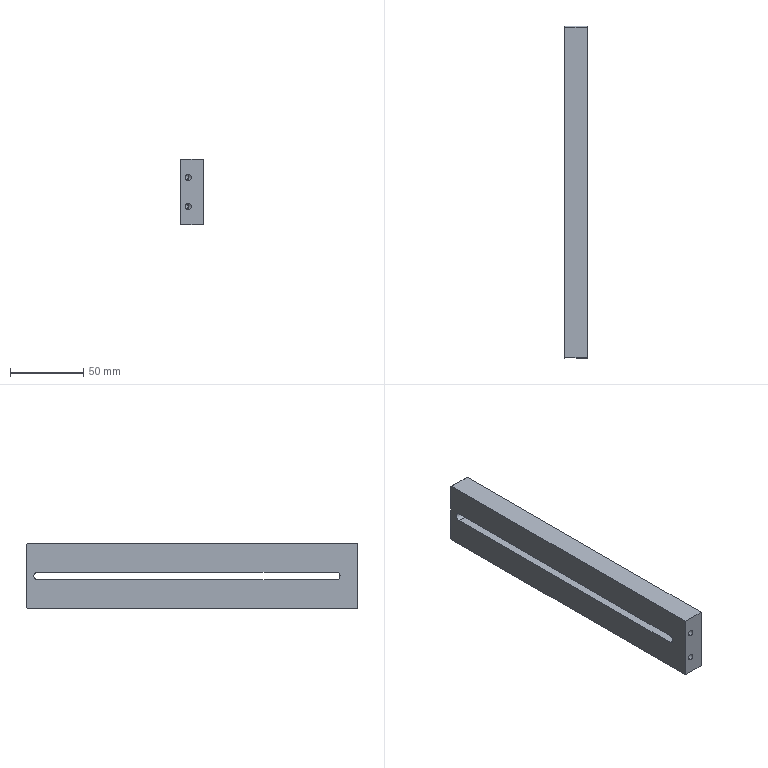Part | SolidWorks | features MoveFace 6, ICE 2, HoleWzd 1, SplitBody 1 | 1 solid | 25 faces | box 15 x 226 x 44.6 mm | volume 129976 mm3 | plane 13 | cylinder 8 | cone 4 | commonest cylinder face diameters 4.2 x4 5.4 x3 9 x1
STEP:
#1=CARTESIAN_POINT('',(-20.,26.4,32.1));
#2=VERTEX_POINT('',#1);
#3=CARTESIAN_POINT('',(-20.,26.4,27.9));
#4=VERTEX_POINT('',#3);
#5=CARTESIAN_POINT('',(-20.,26.4,30.));
#6=DIRECTION('',(0.,-1.,0.));
#7=DIRECTION('',(0.,0.,-1.));
#8=AXIS2_PLACEMENT_3D('',#5,#6,#7);
#9=CIRCLE('',#8,2.1);
#10=EDGE_CURVE('',#2,#4,#9,.T.);
#11=ORIENTED_EDGE('',*,*,#10,.F.);
#12=CARTESIAN_POINT('',(-20.,14.,32.1));
#13=VERTEX_POINT('',#12);
#14=CARTESIAN_POINT('',(-20.,14.,32.1));
#15=DIRECTION('',(0.,-1.,0.));
#16=VECTOR('',#15,1000.);
#17=LINE('',#14,#16);
#18=EDGE_CURVE('',#2,#13,#17,.T.);
#19=ORIENTED_EDGE('',*,*,#18,.T.);
#20=CARTESIAN_POINT('',(-20.,14.,27.9));
#21=VERTEX_POINT('',#20);
#22=CARTESIAN_POINT('',(-20.,14.,30.));
#23=DIRECTION('',(0.,-1.,0.));
#24=DIRECTION('',(0.,0.,-1.));
#25=AXIS2_PLACEMENT_3D('',#22,#23,#24);
#26=CIRCLE('',#25,2.1);
#27=EDGE_CURVE('',#13,#21,#26,.T.);
#28=ORIENTED_EDGE('',*,*,#27,.T.);
#29=CARTESIAN_POINT('',(-20.,14.,27.9));
#30=DIRECTION('',(0.,-1.,0.));
#31=VECTOR('',#30,1000.);
#32=LINE('',#29,#31);
#33=EDGE_CURVE('',#4,#21,#32,.T.);
#34=ORIENTED_EDGE('',*,*,#33,.F.);
#35=EDGE_LOOP('',(#11,#19,#28,#34));
#36=FACE_OUTER_BOUND('',#35,.T.);
#37=CARTESIAN_POINT('',(-20.,14.,30.));
#38=DIRECTION('',(0.,-1.,0.));
#39=DIRECTION('',(0.,0.,-1.));
#40=AXIS2_PLACEMENT_3D('',#37,#38,#39);
#41=CYLINDRICAL_SURFACE('',#40,2.1);
#42=ADVANCED_FACE('',(#36),#41,.F.);
#43=CARTESIAN_POINT('',(-20.,27.662,30.));
#44=VERTEX_POINT('',#43);
#45=CARTESIAN_POINT('',(-20.,26.4,27.9));
#46=DIRECTION('',(0.,-0.515,-0.8572));
#47=VECTOR('',#46,1000.);
#48=LINE('',#45,#47);
#49=EDGE_CURVE('',#44,#4,#48,.T.);
#50=ORIENTED_EDGE('',*,*,#49,.F.);
#51=CARTESIAN_POINT('',(-20.,26.4,32.1));
#52=DIRECTION('',(0.,-0.515,0.8572));
#53=VECTOR('',#52,1000.);
#54=LINE('',#51,#53);
#55=EDGE_CURVE('',#44,#2,#54,.T.);
#56=ORIENTED_EDGE('',*,*,#55,.T.);
#57=ORIENTED_EDGE('',*,*,#10,.T.);
#58=EDGE_LOOP('',(#50,#56,#57));
#59=FACE_OUTER_BOUND('',#58,.T.);
#60=CARTESIAN_POINT('',(-20.,26.4,30.));
#61=DIRECTION('',(0.,-1.,0.));
#62=DIRECTION('',(0.,0.,-1.));
#63=AXIS2_PLACEMENT_3D('',#60,#61,#62);
#64=CONICAL_SURFACE('',#63,2.1,1.03);
#65=ADVANCED_FACE('',(#59),#64,.F.);
#66=CARTESIAN_POINT('',(-20.,26.4,12.1));
#67=VERTEX_POINT('',#66);
#68=CARTESIAN_POINT('',(-20.,26.4,7.9));
#69=VERTEX_POINT('',#68);
#70=CARTESIAN_POINT('',(-20.,26.4,10.));
#71=DIRECTION('',(0.,-1.,0.));
#72=DIRECTION('',(0.,0.,-1.));
#73=AXIS2_PLACEMENT_3D('',#70,#71,#72);
#74=CIRCLE('',#73,2.1);
#75=EDGE_CURVE('',#67,#69,#74,.T.);
#76=ORIENTED_EDGE('',*,*,#75,.F.);
#77=CARTESIAN_POINT('',(-20.,14.,12.1));
#78=VERTEX_POINT('',#77);
#79=CARTESIAN_POINT('',(-20.,14.,12.1));
#80=DIRECTION('',(0.,-1.,0.));
#81=VECTOR('',#80,1000.);
#82=LINE('',#79,#81);
#83=EDGE_CURVE('',#67,#78,#82,.T.);
#84=ORIENTED_EDGE('',*,*,#83,.T.);
#85=CARTESIAN_POINT('',(-20.,14.,7.9));
#86=VERTEX_POINT('',#85);
#87=CARTESIAN_POINT('',(-20.,14.,10.));
#88=DIRECTION('',(0.,-1.,0.));
#89=DIRECTION('',(0.,0.,-1.));
#90=AXIS2_PLACEMENT_3D('',#87,#88,#89);
#91=CIRCLE('',#90,2.1);
#92=EDGE_CURVE('',#78,#86,#91,.T.);
#93=ORIENTED_EDGE('',*,*,#92,.T.);
#94=CARTESIAN_POINT('',(-20.,14.,7.9));
#95=DIRECTION('',(0.,-1.,0.));
#96=VECTOR('',#95,1000.);
#97=LINE('',#94,#96);
#98=EDGE_CURVE('',#69,#86,#97,.T.);
#99=ORIENTED_EDGE('',*,*,#98,.F.);
#100=EDGE_LOOP('',(#76,#84,#93,#99));
#101=FACE_OUTER_BOUND('',#100,.T.);
#102=CARTESIAN_POINT('',(-20.,14.,10.));
#103=DIRECTION('',(0.,-1.,0.));
#104=DIRECTION('',(0.,0.,-1.));
#105=AXIS2_PLACEMENT_3D('',#102,#103,#104);
#106=CYLINDRICAL_SURFACE('',#105,2.1);
#107=ADVANCED_FACE('',(#101),#106,.F.);
#108=CARTESIAN_POINT('',(-20.,27.662,10.));
#109=VERTEX_POINT('',#108);
#110=CARTESIAN_POINT('',(-20.,26.4,7.9));
#111=DIRECTION('',(0.,-0.515,-0.8572));
#112=VECTOR('',#111,1000.);
#113=LINE('',#110,#112);
#114=EDGE_CURVE('',#109,#69,#113,.T.);
#115=ORIENTED_EDGE('',*,*,#114,.F.);
#116=CARTESIAN_POINT('',(-20.,26.4,12.1));
#117=DIRECTION('',(0.,-0.515,0.8572));
#118=VECTOR('',#117,1000.);
#119=LINE('',#116,#118);
#120=EDGE_CURVE('',#109,#67,#119,.T.);
#121=ORIENTED_EDGE('',*,*,#120,.T.);
#122=ORIENTED_EDGE('',*,*,#75,.T.);
#123=EDGE_LOOP('',(#115,#121,#122));
#124=FACE_OUTER_BOUND('',#123,.T.);
#125=CARTESIAN_POINT('',(-20.,26.4,10.));
#126=DIRECTION('',(0.,-1.,0.));
#127=DIRECTION('',(0.,0.,-1.));
#128=AXIS2_PLACEMENT_3D('',#125,#126,#127);
#129=CONICAL_SURFACE('',#128,2.1,1.03);
#130=ADVANCED_FACE('',(#124),#129,.F.);
#131=CARTESIAN_POINT('',(-15.,26.2,20.));
#132=VERTEX_POINT('',#131);
#133=CARTESIAN_POINT('',(-15.,28.9,22.7));
#134=VERTEX_POINT('',#133);
#135=CARTESIAN_POINT('',(-15.,28.9,20.));
#136=DIRECTION('',(-1.,0.,0.));
#137=DIRECTION('',(0.,0.,-1.));
#138=AXIS2_PLACEMENT_3D('',#135,#136,#137);
#139=CIRCLE('',#138,2.7);
#140=EDGE_CURVE('',#132,#134,#139,.T.);
#141=ORIENTED_EDGE('',*,*,#140,.F.);
#142=CARTESIAN_POINT('',(-25.,26.2,20.));
#143=VERTEX_POINT('',#142);
#144=CARTESIAN_POINT('',(5.,26.2,20.));
#145=DIRECTION('',(-1.,0.,0.));
#146=VECTOR('',#145,1000.);
#147=LINE('',#144,#146);
#148=EDGE_CURVE('',#132,#143,#147,.T.);
#149=ORIENTED_EDGE('',*,*,#148,.T.);
#150=CARTESIAN_POINT('',(-25.,28.9,22.7));
#151=VERTEX_POINT('',#150);
#152=CARTESIAN_POINT('',(-25.,28.9,20.));
#153=DIRECTION('',(-1.,0.,0.));
#154=DIRECTION('',(0.,-1.,0.));
#155=AXIS2_PLACEMENT_3D('',#152,#153,#154);
#156=CIRCLE('',#155,2.7);
#157=EDGE_CURVE('',#143,#151,#156,.T.);
#158=ORIENTED_EDGE('',*,*,#157,.T.);
#159=CARTESIAN_POINT('',(5.,28.9,22.7));
#160=DIRECTION('',(-1.,0.,0.));
#161=VECTOR('',#160,1000.);
#162=LINE('',#159,#161);
#163=EDGE_CURVE('',#134,#151,#162,.T.);
#164=ORIENTED_EDGE('',*,*,#163,.F.);
#165=EDGE_LOOP('',(#141,#149,#158,#164));
#166=FACE_OUTER_BOUND('',#165,.T.);
#167=CARTESIAN_POINT('',(5.,28.9,20.));
#168=DIRECTION('',(-1.,0.,0.));
#169=DIRECTION('',(0.,-1.,0.));
#170=AXIS2_PLACEMENT_3D('',#167,#168,#169);
#171=CYLINDRICAL_SURFACE('',#170,2.7);
#172=ADVANCED_FACE('',(#166),#171,.F.);
#173=CARTESIAN_POINT('',(-20.,14.,30.));
#174=DIRECTION('',(0.,-1.,0.));
#175=DIRECTION('',(0.,0.,-1.));
#176=AXIS2_PLACEMENT_3D('',#173,#174,#175);
#177=CIRCLE('',#176,2.1);
#178=EDGE_CURVE('',#21,#13,#177,.T.);
#179=ORIENTED_EDGE('',*,*,#178,.F.);
#180=ORIENTED_EDGE('',*,*,#27,.F.);
#181=EDGE_LOOP('',(#179,#180));
#182=FACE_BOUND('',#181,.T.);
#183=CARTESIAN_POINT('',(-20.,14.,10.));
#184=DIRECTION('',(0.,-1.,0.));
#185=DIRECTION('',(0.,0.,-1.));
#186=AXIS2_PLACEMENT_3D('',#183,#184,#185);
#187=CIRCLE('',#186,2.1);
#188=EDGE_CURVE('',#86,#78,#187,.T.);
#189=ORIENTED_EDGE('',*,*,#188,.F.);
#190=ORIENTED_EDGE('',*,*,#92,.F.);
#191=EDGE_LOOP('',(#189,#190));
#192=FACE_BOUND('',#191,.T.);
#193=CARTESIAN_POINT('',(-25.,14.,-2.3));
#194=VERTEX_POINT('',#193);
#195=CARTESIAN_POINT('',(-25.,14.,42.3));
#196=VERTEX_POINT('',#195);
#197=CARTESIAN_POINT('',(-25.,14.,40.));
#198=DIRECTION('',(0.,0.,1.));
#199=VECTOR('',#198,1000.);
#200=LINE('',#197,#199);
#201=EDGE_CURVE('',#194,#196,#200,.T.);
#202=ORIENTED_EDGE('',*,*,#201,.F.);
#203=CARTESIAN_POINT('',(-10.,14.,-2.3));
#204=VERTEX_POINT('',#203);
#205=CARTESIAN_POINT('',(-5.,14.,-2.3));
#206=DIRECTION('',(1.,0.,0.));
#207=VECTOR('',#206,1000.);
#208=LINE('',#205,#207);
#209=EDGE_CURVE('',#194,#204,#208,.T.);
#210=ORIENTED_EDGE('',*,*,#209,.T.);
#211=CARTESIAN_POINT('',(-10.,14.,42.3));
#212=VERTEX_POINT('',#211);
#213=CARTESIAN_POINT('',(-10.,14.,40.));
#214=DIRECTION('',(0.,0.,1.));
#215=VECTOR('',#214,1000.);
#216=LINE('',#213,#215);
#217=EDGE_CURVE('',#204,#212,#216,.T.);
#218=ORIENTED_EDGE('',*,*,#217,.T.);
#219=CARTESIAN_POINT('',(-5.,14.,42.3));
#220=DIRECTION('',(-1.,0.,0.));
#221=VECTOR('',#220,1000.);
#222=LINE('',#219,#221);
#223=EDGE_CURVE('',#212,#196,#222,.T.);
#224=ORIENTED_EDGE('',*,*,#223,.T.);
#225=EDGE_LOOP('',(#202,#210,#218,#224));
#226=FACE_OUTER_BOUND('',#225,.T.);
#227=CARTESIAN_POINT('',(-5.,14.,40.));
#228=DIRECTION('',(0.,1.,0.));
#229=DIRECTION('',(0.,0.,1.));
#230=AXIS2_PLACEMENT_3D('',#227,#228,#229);
#231=PLANE('',#230);
#232=ADVANCED_FACE('',(#182,#192,#226),#231,.F.);
#233=CARTESIAN_POINT('',(-25.,232.,22.7));
#234=VERTEX_POINT('',#233);
#235=CARTESIAN_POINT('',(-25.,18.9,22.7));
#236=DIRECTION('',(0.,1.,0.));
#237=VECTOR('',#236,1000.);
#238=LINE('',#235,#237);
#239=EDGE_CURVE('',#151,#234,#238,.T.);
#240=ORIENTED_EDGE('',*,*,#239,.F.);
#241=ORIENTED_EDGE('',*,*,#157,.F.);
#242=CARTESIAN_POINT('',(-25.,28.9,17.3));
#243=VERTEX_POINT('',#242);
#244=CARTESIAN_POINT('',(-25.,28.9,20.));
#245=DIRECTION('',(-1.,0.,0.));
#246=DIRECTION('',(0.,-1.,0.));
#247=AXIS2_PLACEMENT_3D('',#244,#245,#246);
#248=CIRCLE('',#247,2.7);
#249=EDGE_CURVE('',#243,#143,#248,.T.);
#250=ORIENTED_EDGE('',*,*,#249,.F.);
#251=CARTESIAN_POINT('',(-25.,232.,17.3));
#252=VERTEX_POINT('',#251);
#253=CARTESIAN_POINT('',(-25.,18.9,17.3));
#254=DIRECTION('',(0.,-1.,0.));
#255=VECTOR('',#254,1000.);
#256=LINE('',#253,#255);
#257=EDGE_CURVE('',#252,#243,#256,.T.);
#258=ORIENTED_EDGE('',*,*,#257,.F.);
#259=CARTESIAN_POINT('',(-25.,232.,20.));
#260=DIRECTION('',(-1.,0.,0.));
#261=DIRECTION('',(0.,-1.,0.));
#262=AXIS2_PLACEMENT_3D('',#259,#260,#261);
#263=CIRCLE('',#262,2.7);
#264=EDGE_CURVE('',#234,#252,#263,.T.);
#265=ORIENTED_EDGE('',*,*,#264,.F.);
#266=EDGE_LOOP('',(#240,#241,#250,#258,#265));
#267=FACE_BOUND('',#266,.T.);
#268=CARTESIAN_POINT('',(-25.,239.3,-2.3));
#269=VERTEX_POINT('',#268);
#270=CARTESIAN_POINT('',(-25.,200.,-2.3));
#271=DIRECTION('',(0.,-1.,0.));
#272=VECTOR('',#271,1000.);
#273=LINE('',#270,#272);
#274=EDGE_CURVE('',#269,#194,#273,.T.);
#275=ORIENTED_EDGE('',*,*,#274,.T.);
#276=ORIENTED_EDGE('',*,*,#201,.T.);
#277=CARTESIAN_POINT('',(-25.,239.3,42.3));
#278=VERTEX_POINT('',#277);
#279=CARTESIAN_POINT('',(-25.,200.,42.3));
#280=DIRECTION('',(0.,1.,0.));
#281=VECTOR('',#280,1000.);
#282=LINE('',#279,#281);
#283=EDGE_CURVE('',#196,#278,#282,.T.);
#284=ORIENTED_EDGE('',*,*,#283,.T.);
#285=CARTESIAN_POINT('',(-25.,240.,41.6));
#286=VERTEX_POINT('',#285);
#287=CARTESIAN_POINT('',(-25.,237.,44.6));
#288=DIRECTION('',(0.,0.7071,-0.7071));
#289=VECTOR('',#288,1000.);
#290=LINE('',#287,#289);
#291=EDGE_CURVE('',#278,#286,#290,.T.);
#292=ORIENTED_EDGE('',*,*,#291,.T.);
#293=CARTESIAN_POINT('',(-25.,240.,-1.6));
#294=VERTEX_POINT('',#293);
#295=CARTESIAN_POINT('',(-25.,240.,40.));
#296=DIRECTION('',(0.,0.,-1.));
#297=VECTOR('',#296,1000.);
#298=LINE('',#295,#297);
#299=EDGE_CURVE('',#286,#294,#298,.T.);
#300=ORIENTED_EDGE('',*,*,#299,.T.);
#301=CARTESIAN_POINT('',(-25.,240.,-1.6));
#302=DIRECTION('',(0.,-0.7071,-0.7071));
#303=VECTOR('',#302,1000.);
#304=LINE('',#301,#303);
#305=EDGE_CURVE('',#294,#269,#304,.T.);
#306=ORIENTED_EDGE('',*,*,#305,.T.);
#307=EDGE_LOOP('',(#275,#276,#284,#292,#300,#306));
#308=FACE_OUTER_BOUND('',#307,.T.);
#309=CARTESIAN_POINT('',(-25.,200.,40.));
#310=DIRECTION('',(1.,0.,0.));
#311=DIRECTION('',(0.,1.,0.));
#312=AXIS2_PLACEMENT_3D('',#309,#310,#311);
#313=PLANE('',#312);
#314=ADVANCED_FACE('',(#267,#308),#313,.F.);
#315=CARTESIAN_POINT('',(-15.,232.,22.7));
#316=VERTEX_POINT('',#315);
#317=CARTESIAN_POINT('',(-15.,18.9,22.7));
#318=DIRECTION('',(0.,1.,0.));
#319=VECTOR('',#318,1000.);
#320=LINE('',#317,#319);
#321=EDGE_CURVE('',#134,#316,#320,.T.);
#322=ORIENTED_EDGE('',*,*,#321,.F.);
#323=ORIENTED_EDGE('',*,*,#163,.T.);
#324=ORIENTED_EDGE('',*,*,#239,.T.);
#325=CARTESIAN_POINT('',(5.,232.,22.7));
#326=DIRECTION('',(-1.,0.,0.));
#327=VECTOR('',#326,1000.);
#328=LINE('',#325,#327);
#329=EDGE_CURVE('',#316,#234,#328,.T.);
#330=ORIENTED_EDGE('',*,*,#329,.F.);
#331=EDGE_LOOP('',(#322,#323,#324,#330));
#332=FACE_OUTER_BOUND('',#331,.T.);
#333=CARTESIAN_POINT('',(5.,18.9,22.7));
#334=DIRECTION('',(0.,0.,1.));
#335=DIRECTION('',(1.,0.,0.));
#336=AXIS2_PLACEMENT_3D('',#333,#334,#335);
#337=PLANE('',#336);
#338=ADVANCED_FACE('',(#332),#337,.F.);
#339=ORIENTED_EDGE('',*,*,#148,.F.);
#340=CARTESIAN_POINT('',(-15.,28.9,17.3));
#341=VERTEX_POINT('',#340);
#342=CARTESIAN_POINT('',(-15.,28.9,20.));
#343=DIRECTION('',(-1.,0.,0.));
#344=DIRECTION('',(0.,0.,-1.));
#345=AXIS2_PLACEMENT_3D('',#342,#343,#344);
#346=CIRCLE('',#345,2.7);
#347=EDGE_CURVE('',#341,#132,#346,.T.);
#348=ORIENTED_EDGE('',*,*,#347,.F.);
#349=CARTESIAN_POINT('',(5.,28.9,17.3));
#350=DIRECTION('',(-1.,0.,0.));
#351=VECTOR('',#350,1000.);
#352=LINE('',#349,#351);
#353=EDGE_CURVE('',#341,#243,#352,.T.);
#354=ORIENTED_EDGE('',*,*,#353,.T.);
#355=ORIENTED_EDGE('',*,*,#249,.T.);
#356=EDGE_LOOP('',(#339,#348,#354,#355));
#357=FACE_OUTER_BOUND('',#356,.T.);
#358=CARTESIAN_POINT('',(5.,28.9,20.));
#359=DIRECTION('',(-1.,0.,0.));
#360=DIRECTION('',(0.,-1.,0.));
#361=AXIS2_PLACEMENT_3D('',#358,#359,#360);
#362=CYLINDRICAL_SURFACE('',#361,2.7);
#363=ADVANCED_FACE('',(#357),#362,.F.);
#364=CARTESIAN_POINT('',(-15.,232.,17.3));
#365=VERTEX_POINT('',#364);
#366=CARTESIAN_POINT('',(-15.,18.9,17.3));
#367=DIRECTION('',(0.,-1.,0.));
#368=VECTOR('',#367,1000.);
#369=LINE('',#366,#368);
#370=EDGE_CURVE('',#365,#341,#369,.T.);
#371=ORIENTED_EDGE('',*,*,#370,.F.);
#372=CARTESIAN_POINT('',(5.,232.,17.3));
#373=DIRECTION('',(-1.,0.,0.));
#374=VECTOR('',#373,1000.);
#375=LINE('',#372,#374);
#376=EDGE_CURVE('',#365,#252,#375,.T.);
#377=ORIENTED_EDGE('',*,*,#376,.T.);
#378=ORIENTED_EDGE('',*,*,#257,.T.);
#379=ORIENTED_EDGE('',*,*,#353,.F.);
#380=EDGE_LOOP('',(#371,#377,#378,#379));
#381=FACE_OUTER_BOUND('',#380,.T.);
#382=CARTESIAN_POINT('',(5.,18.9,17.3));
#383=DIRECTION('',(0.,0.,-1.));
#384=DIRECTION('',(-1.,0.,0.));
#385=AXIS2_PLACEMENT_3D('',#382,#383,#384);
#386=PLANE('',#385);
#387=ADVANCED_FACE('',(#381),#386,.F.);
#388=CARTESIAN_POINT('',(-15.,232.,20.));
#389=DIRECTION('',(-1.,0.,0.));
#390=DIRECTION('',(0.,0.,-1.));
#391=AXIS2_PLACEMENT_3D('',#388,#389,#390);
#392=CIRCLE('',#391,2.7);
#393=EDGE_CURVE('',#316,#365,#392,.T.);
#394=ORIENTED_EDGE('',*,*,#393,.F.);
#395=ORIENTED_EDGE('',*,*,#329,.T.);
#396=ORIENTED_EDGE('',*,*,#264,.T.);
#397=ORIENTED_EDGE('',*,*,#376,.F.);
#398=EDGE_LOOP('',(#394,#395,#396,#397));
#399=FACE_OUTER_BOUND('',#398,.T.);
#400=CARTESIAN_POINT('',(5.,232.,20.));
#401=DIRECTION('',(-1.,0.,0.));
#402=DIRECTION('',(0.,-1.,0.));
#403=AXIS2_PLACEMENT_3D('',#400,#401,#402);
#404=CYLINDRICAL_SURFACE('',#403,2.7);
#405=ADVANCED_FACE('',(#399),#404,.F.);
#406=ORIENTED_EDGE('',*,*,#223,.F.);
#407=CARTESIAN_POINT('',(-10.,239.3,42.3));
#408=VERTEX_POINT('',#407);
#409=CARTESIAN_POINT('',(-10.,-6.,42.3));
#410=DIRECTION('',(0.,-1.,0.));
#411=VECTOR('',#410,1000.);
#412=LINE('',#409,#411);
#413=EDGE_CURVE('',#408,#212,#412,.T.);
#414=ORIENTED_EDGE('',*,*,#413,.F.);
#415=CARTESIAN_POINT('',(0.,239.3,42.3));
#416=DIRECTION('',(-1.,0.,0.));
#417=VECTOR('',#416,1000.);
#418=LINE('',#415,#417);
#419=EDGE_CURVE('',#408,#278,#418,.T.);
#420=ORIENTED_EDGE('',*,*,#419,.T.);
#421=ORIENTED_EDGE('',*,*,#283,.F.);
#422=EDGE_LOOP('',(#406,#414,#420,#421));
#423=FACE_OUTER_BOUND('',#422,.T.);
#424=CARTESIAN_POINT('',(-65.,209.601,42.3));
#425=DIRECTION('',(0.,0.,-1.));
#426=DIRECTION('',(0.,1.,0.));
#427=AXIS2_PLACEMENT_3D('',#424,#425,#426);
#428=PLANE('',#427);
#429=ADVANCED_FACE('',(#423),#428,.F.);
#430=CARTESIAN_POINT('',(-10.,240.,41.6));
#431=VERTEX_POINT('',#430);
#432=CARTESIAN_POINT('',(-10.,237.,44.6));
#433=DIRECTION('',(0.,-0.7071,0.7071));
#434=VECTOR('',#433,1000.);
#435=LINE('',#432,#434);
#436=EDGE_CURVE('',#431,#408,#435,.T.);
#437=ORIENTED_EDGE('',*,*,#436,.F.);
#438=CARTESIAN_POINT('',(0.,240.,41.6));
#439=DIRECTION('',(1.,0.,0.));
#440=VECTOR('',#439,1000.);
#441=LINE('',#438,#440);
#442=EDGE_CURVE('',#286,#431,#441,.T.);
#443=ORIENTED_EDGE('',*,*,#442,.F.);
#444=ORIENTED_EDGE('',*,*,#291,.F.);
#445=ORIENTED_EDGE('',*,*,#419,.F.);
#446=EDGE_LOOP('',(#437,#443,#444,#445));
#447=FACE_OUTER_BOUND('',#446,.T.);
#448=CARTESIAN_POINT('',(0.,237.,44.6));
#449=DIRECTION('',(0.,0.7071,0.7071));
#450=DIRECTION('',(1.,0.,0.));
#451=AXIS2_PLACEMENT_3D('',#448,#449,#450);
#452=PLANE('',#451);
#453=ADVANCED_FACE('',(#447),#452,.T.);
#454=CARTESIAN_POINT('',(-15.,240.,15.5));
#455=VERTEX_POINT('',#454);
#456=CARTESIAN_POINT('',(-15.,240.,24.5));
#457=VERTEX_POINT('',#456);
#458=CARTESIAN_POINT('',(-15.,240.,40.));
#459=DIRECTION('',(0.,0.,1.));
#460=VECTOR('',#459,1000.);
#461=LINE('',#458,#460);
#462=EDGE_CURVE('',#455,#457,#461,.T.);
#463=ORIENTED_EDGE('',*,*,#462,.F.);
#464=CARTESIAN_POINT('',(-10.,240.,15.5));
#465=VERTEX_POINT('',#464);
#466=CARTESIAN_POINT('',(-15.,240.,15.5));
#467=DIRECTION('',(1.,0.,0.));
#468=VECTOR('',#467,1000.);
#469=LINE('',#466,#468);
#470=EDGE_CURVE('',#455,#465,#469,.T.);
#471=ORIENTED_EDGE('',*,*,#470,.T.);
#472=CARTESIAN_POINT('',(-10.,240.,-1.6));
#473=VERTEX_POINT('',#472);
#474=CARTESIAN_POINT('',(-10.,240.,40.));
#475=DIRECTION('',(0.,0.,-1.));
#476=VECTOR('',#475,1000.);
#477=LINE('',#474,#476);
#478=EDGE_CURVE('',#465,#473,#477,.T.);
#479=ORIENTED_EDGE('',*,*,#478,.T.);
#480=CARTESIAN_POINT('',(0.,240.,-1.6));
#481=DIRECTION('',(-1.,0.,0.));
#482=VECTOR('',#481,1000.);
#483=LINE('',#480,#482);
#484=EDGE_CURVE('',#473,#294,#483,.T.);
#485=ORIENTED_EDGE('',*,*,#484,.T.);
#486=ORIENTED_EDGE('',*,*,#299,.F.);
#487=ORIENTED_EDGE('',*,*,#442,.T.);
#488=CARTESIAN_POINT('',(-10.,240.,24.5));
#489=VERTEX_POINT('',#488);
#490=CARTESIAN_POINT('',(-10.,240.,40.));
#491=DIRECTION('',(0.,0.,-1.));
#492=VECTOR('',#491,1000.);
#493=LINE('',#490,#492);
#494=EDGE_CURVE('',#431,#489,#493,.T.);
#495=ORIENTED_EDGE('',*,*,#494,.T.);
#496=CARTESIAN_POINT('',(-15.,240.,24.5));
#497=DIRECTION('',(1.,0.,0.));
#498=VECTOR('',#497,1000.);
#499=LINE('',#496,#498);
#500=EDGE_CURVE('',#457,#489,#499,.T.);
#501=ORIENTED_EDGE('',*,*,#500,.F.);
#502=EDGE_LOOP('',(#463,#471,#479,#485,#486,#487,#495,#501));
#503=FACE_OUTER_BOUND('',#502,.T.);
#504=CARTESIAN_POINT('',(0.,240.,40.));
#505=DIRECTION('',(0.,-1.,0.));
#506=DIRECTION('',(0.,0.,-1.));
#507=AXIS2_PLACEMENT_3D('',#504,#505,#506);
#508=PLANE('',#507);
#509=ADVANCED_FACE('',(#503),#508,.F.);
#510=CARTESIAN_POINT('',(-10.,239.3,-2.3));
#511=VERTEX_POINT('',#510);
#512=CARTESIAN_POINT('',(-10.,240.,-1.6));
#513=DIRECTION('',(0.,0.7071,0.7071));
#514=VECTOR('',#513,1000.);
#515=LINE('',#512,#514);
#516=EDGE_CURVE('',#511,#473,#515,.T.);
#517=ORIENTED_EDGE('',*,*,#516,.F.);
#518=CARTESIAN_POINT('',(0.,239.3,-2.3));
#519=DIRECTION('',(1.,0.,0.));
#520=VECTOR('',#519,1000.);
#521=LINE('',#518,#520);
#522=EDGE_CURVE('',#269,#511,#521,.T.);
#523=ORIENTED_EDGE('',*,*,#522,.F.);
#524=ORIENTED_EDGE('',*,*,#305,.F.);
#525=ORIENTED_EDGE('',*,*,#484,.F.);
#526=EDGE_LOOP('',(#517,#523,#524,#525));
#527=FACE_OUTER_BOUND('',#526,.T.);
#528=CARTESIAN_POINT('',(0.,240.,-1.6));
#529=DIRECTION('',(0.,-0.7071,0.7071));
#530=DIRECTION('',(-1.,0.,0.));
#531=AXIS2_PLACEMENT_3D('',#528,#529,#530);
#532=PLANE('',#531);
#533=ADVANCED_FACE('',(#527),#532,.F.);
#534=ORIENTED_EDGE('',*,*,#522,.T.);
#535=CARTESIAN_POINT('',(-10.,-6.,-2.3));
#536=DIRECTION('',(0.,-1.,0.));
#537=VECTOR('',#536,1000.);
#538=LINE('',#535,#537);
#539=EDGE_CURVE('',#511,#204,#538,.T.);
#540=ORIENTED_EDGE('',*,*,#539,.T.);
#541=ORIENTED_EDGE('',*,*,#209,.F.);
#542=ORIENTED_EDGE('',*,*,#274,.F.);
#543=EDGE_LOOP('',(#534,#540,#541,#542));
#544=FACE_OUTER_BOUND('',#543,.T.);
#545=CARTESIAN_POINT('',(-65.,209.601,-2.3));
#546=DIRECTION('',(0.,0.,1.));
#547=DIRECTION('',(0.,-1.,0.));
#548=AXIS2_PLACEMENT_3D('',#545,#546,#547);
#549=PLANE('',#548);
#550=ADVANCED_FACE('',(#544),#549,.F.);
#551=ORIENTED_EDGE('',*,*,#478,.F.);
#552=CARTESIAN_POINT('',(-10.,28.9,15.5));
#553=VERTEX_POINT('',#552);
#554=CARTESIAN_POINT('',(-10.,18.9,15.5));
#555=DIRECTION('',(0.,1.,0.));
#556=VECTOR('',#555,1000.);
#557=LINE('',#554,#556);
#558=EDGE_CURVE('',#553,#465,#557,.T.);
#559=ORIENTED_EDGE('',*,*,#558,.F.);
#560=CARTESIAN_POINT('',(-10.,28.9,24.5));
#561=VERTEX_POINT('',#560);
#562=CARTESIAN_POINT('',(-10.,28.9,20.));
#563=DIRECTION('',(1.,0.,0.));
#564=DIRECTION('',(0.,0.,1.));
#565=AXIS2_PLACEMENT_3D('',#562,#563,#564);
#566=CIRCLE('',#565,4.5);
#567=EDGE_CURVE('',#561,#553,#566,.T.);
#568=ORIENTED_EDGE('',*,*,#567,.F.);
#569=CARTESIAN_POINT('',(-10.,18.9,24.5));
#570=DIRECTION('',(0.,-1.,0.));
#571=VECTOR('',#570,1000.);
#572=LINE('',#569,#571);
#573=EDGE_CURVE('',#489,#561,#572,.T.);
#574=ORIENTED_EDGE('',*,*,#573,.F.);
#575=ORIENTED_EDGE('',*,*,#494,.F.);
#576=ORIENTED_EDGE('',*,*,#436,.T.);
#577=ORIENTED_EDGE('',*,*,#413,.T.);
#578=ORIENTED_EDGE('',*,*,#217,.F.);
#579=ORIENTED_EDGE('',*,*,#539,.F.);
#580=ORIENTED_EDGE('',*,*,#516,.T.);
#581=EDGE_LOOP('',(#551,#559,#568,#574,#575,#576,#577,#578,#579,#580));
#582=FACE_OUTER_BOUND('',#581,.T.);
#583=CARTESIAN_POINT('',(-10.,-6.,2.3));
#584=DIRECTION('',(-1.,0.,0.));
#585=DIRECTION('',(0.,0.,1.));
#586=AXIS2_PLACEMENT_3D('',#583,#584,#585);
#587=PLANE('',#586);
#588=ADVANCED_FACE('',(#582),#587,.F.);
#589=ORIENTED_EDGE('',*,*,#321,.T.);
#590=ORIENTED_EDGE('',*,*,#393,.T.);
#591=ORIENTED_EDGE('',*,*,#370,.T.);
#592=ORIENTED_EDGE('',*,*,#347,.T.);
#593=ORIENTED_EDGE('',*,*,#140,.T.);
#594=EDGE_LOOP('',(#589,#590,#591,#592,#593));
#595=FACE_BOUND('',#594,.T.);
#596=ORIENTED_EDGE('',*,*,#462,.T.);
#597=CARTESIAN_POINT('',(-15.,28.9,24.5));
#598=VERTEX_POINT('',#597);
#599=CARTESIAN_POINT('',(-15.,18.9,24.5));
#600=DIRECTION('',(0.,-1.,0.));
#601=VECTOR('',#600,1000.);
#602=LINE('',#599,#601);
#603=EDGE_CURVE('',#457,#598,#602,.T.);
#604=ORIENTED_EDGE('',*,*,#603,.T.);
#605=CARTESIAN_POINT('',(-15.,28.9,15.5));
#606=VERTEX_POINT('',#605);
#607=CARTESIAN_POINT('',(-15.,28.9,20.));
#608=DIRECTION('',(1.,0.,0.));
#609=DIRECTION('',(0.,0.,-1.));
#610=AXIS2_PLACEMENT_3D('',#607,#608,#609);
#611=CIRCLE('',#610,4.5);
#612=EDGE_CURVE('',#598,#606,#611,.T.);
#613=ORIENTED_EDGE('',*,*,#612,.T.);
#614=CARTESIAN_POINT('',(-15.,18.9,15.5));
#615=DIRECTION('',(0.,1.,0.));
#616=VECTOR('',#615,1000.);
#617=LINE('',#614,#616);
#618=EDGE_CURVE('',#606,#455,#617,.T.);
#619=ORIENTED_EDGE('',*,*,#618,.T.);
#620=EDGE_LOOP('',(#596,#604,#613,#619));
#621=FACE_OUTER_BOUND('',#620,.T.);
#622=CARTESIAN_POINT('',(-15.,18.9,20.));
#623=DIRECTION('',(1.,0.,0.));
#624=DIRECTION('',(0.,0.,-1.));
#625=AXIS2_PLACEMENT_3D('',#622,#623,#624);
#626=PLANE('',#625);
#627=ADVANCED_FACE('',(#595,#621),#626,.T.);
#628=CARTESIAN_POINT('',(-15.,28.9,15.5));
#629=DIRECTION('',(1.,0.,0.));
#630=VECTOR('',#629,1000.);
#631=LINE('',#628,#630);
#632=EDGE_CURVE('',#606,#553,#631,.T.);
#633=ORIENTED_EDGE('',*,*,#632,.T.);
#634=ORIENTED_EDGE('',*,*,#558,.T.);
#635=ORIENTED_EDGE('',*,*,#470,.F.);
#636=ORIENTED_EDGE('',*,*,#618,.F.);
#637=EDGE_LOOP('',(#633,#634,#635,#636));
#638=FACE_OUTER_BOUND('',#637,.T.);
#639=CARTESIAN_POINT('',(-15.,18.9,15.5));
#640=DIRECTION('',(0.,0.,-1.));
#641=DIRECTION('',(-1.,0.,0.));
#642=AXIS2_PLACEMENT_3D('',#639,#640,#641);
#643=PLANE('',#642);
#644=ADVANCED_FACE('',(#638),#643,.F.);
#645=ORIENTED_EDGE('',*,*,#603,.F.);
#646=ORIENTED_EDGE('',*,*,#500,.T.);
#647=ORIENTED_EDGE('',*,*,#573,.T.);
#648=CARTESIAN_POINT('',(-15.,28.9,24.5));
#649=DIRECTION('',(1.,0.,0.));
#650=VECTOR('',#649,1000.);
#651=LINE('',#648,#650);
#652=EDGE_CURVE('',#598,#561,#651,.T.);
#653=ORIENTED_EDGE('',*,*,#652,.F.);
#654=EDGE_LOOP('',(#645,#646,#647,#653));
#655=FACE_OUTER_BOUND('',#654,.T.);
#656=CARTESIAN_POINT('',(-15.,18.9,24.5));
#657=DIRECTION('',(0.,0.,1.));
#658=DIRECTION('',(1.,0.,0.));
#659=AXIS2_PLACEMENT_3D('',#656,#657,#658);
#660=PLANE('',#659);
#661=ADVANCED_FACE('',(#655),#660,.F.);
#662=ORIENTED_EDGE('',*,*,#652,.T.);
#663=ORIENTED_EDGE('',*,*,#567,.T.);
#664=ORIENTED_EDGE('',*,*,#632,.F.);
#665=ORIENTED_EDGE('',*,*,#612,.F.);
#666=EDGE_LOOP('',(#662,#663,#664,#665));
#667=FACE_OUTER_BOUND('',#666,.T.);
#668=CARTESIAN_POINT('',(-15.,28.9,20.));
#669=DIRECTION('',(1.,0.,0.));
#670=DIRECTION('',(0.,0.,-1.));
#671=AXIS2_PLACEMENT_3D('',#668,#669,#670);
#672=CYLINDRICAL_SURFACE('',#671,4.5);
#673=ADVANCED_FACE('',(#667),#672,.F.);
#674=ORIENTED_EDGE('',*,*,#120,.F.);
#675=ORIENTED_EDGE('',*,*,#114,.T.);
#676=CARTESIAN_POINT('',(-20.,26.4,10.));
#677=DIRECTION('',(0.,-1.,0.));
#678=DIRECTION('',(0.,0.,-1.));
#679=AXIS2_PLACEMENT_3D('',#676,#677,#678);
#680=CIRCLE('',#679,2.1);
#681=EDGE_CURVE('',#69,#67,#680,.T.);
#682=ORIENTED_EDGE('',*,*,#681,.T.);
#683=EDGE_LOOP('',(#674,#675,#682));
#684=FACE_OUTER_BOUND('',#683,.T.);
#685=CARTESIAN_POINT('',(-20.,26.4,10.));
#686=DIRECTION('',(0.,-1.,0.));
#687=DIRECTION('',(0.,0.,-1.));
#688=AXIS2_PLACEMENT_3D('',#685,#686,#687);
#689=CONICAL_SURFACE('',#688,2.1,1.03);
#690=ADVANCED_FACE('',(#684),#689,.F.);
#691=ORIENTED_EDGE('',*,*,#83,.F.);
#692=ORIENTED_EDGE('',*,*,#681,.F.);
#693=ORIENTED_EDGE('',*,*,#98,.T.);
#694=ORIENTED_EDGE('',*,*,#188,.T.);
#695=EDGE_LOOP('',(#691,#692,#693,#694));
#696=FACE_OUTER_BOUND('',#695,.T.);
#697=CARTESIAN_POINT('',(-20.,14.,10.));
#698=DIRECTION('',(0.,-1.,0.));
#699=DIRECTION('',(0.,0.,-1.));
#700=AXIS2_PLACEMENT_3D('',#697,#698,#699);
#701=CYLINDRICAL_SURFACE('',#700,2.1);
#702=ADVANCED_FACE('',(#696),#701,.F.);
#703=ORIENTED_EDGE('',*,*,#55,.F.);
#704=ORIENTED_EDGE('',*,*,#49,.T.);
#705=CARTESIAN_POINT('',(-20.,26.4,30.));
#706=DIRECTION('',(0.,-1.,0.));
#707=DIRECTION('',(0.,0.,-1.));
#708=AXIS2_PLACEMENT_3D('',#705,#706,#707);
#709=CIRCLE('',#708,2.1);
#710=EDGE_CURVE('',#4,#2,#709,.T.);
#711=ORIENTED_EDGE('',*,*,#710,.T.);
#712=EDGE_LOOP('',(#703,#704,#711));
#713=FACE_OUTER_BOUND('',#712,.T.);
#714=CARTESIAN_POINT('',(-20.,26.4,30.));
#715=DIRECTION('',(0.,-1.,0.));
#716=DIRECTION('',(0.,0.,-1.));
#717=AXIS2_PLACEMENT_3D('',#714,#715,#716);
#718=CONICAL_SURFACE('',#717,2.1,1.03);
#719=ADVANCED_FACE('',(#713),#718,.F.);
#720=ORIENTED_EDGE('',*,*,#18,.F.);
#721=ORIENTED_EDGE('',*,*,#710,.F.);
#722=ORIENTED_EDGE('',*,*,#33,.T.);
#723=ORIENTED_EDGE('',*,*,#178,.T.);
#724=EDGE_LOOP('',(#720,#721,#722,#723));
#725=FACE_OUTER_BOUND('',#724,.T.);
#726=CARTESIAN_POINT('',(-20.,14.,30.));
#727=DIRECTION('',(0.,-1.,0.));
#728=DIRECTION('',(0.,0.,-1.));
#729=AXIS2_PLACEMENT_3D('',#726,#727,#728);
#730=CYLINDRICAL_SURFACE('',#729,2.1);
#731=ADVANCED_FACE('',(#725),#730,.F.);
#732=CLOSED_SHELL('',(#42,#65,#107,#130,#172,#232,#314,#338,#363,#387,#405,#429,#453,#509,#533,#550,#588,#627,#644,#661,#673,#690,#702,#719,#731));
#733=MANIFOLD_SOLID_BREP('',#732);
#734=CARTESIAN_POINT('',(0.,0.,0.));
#735=DIRECTION('',(0.,0.,1.));
#736=DIRECTION('',(1.,0.,0.));
#737=AXIS2_PLACEMENT_3D('',#734,#735,#736);
#738=(LENGTH_UNIT()NAMED_UNIT(*)SI_UNIT(.MILLI.,.METRE.));
#739=UNCERTAINTY_MEASURE_WITH_UNIT(LENGTH_MEASURE(0.00001),#738,'','');
#740=(NAMED_UNIT(*)PLANE_ANGLE_UNIT()SI_UNIT($,.RADIAN.));
#741=(NAMED_UNIT(*)SI_UNIT($,.STERADIAN.)SOLID_ANGLE_UNIT());
#742=(GEOMETRIC_REPRESENTATION_CONTEXT(3)GLOBAL_UNCERTAINTY_ASSIGNED_CONTEXT((#739))GLOBAL_UNIT_ASSIGNED_CONTEXT((#738,#740,#741))REPRESENTATION_CONTEXT('',''));
#743=ADVANCED_BREP_SHAPE_REPRESENTATION('',(#733,#737),#742);